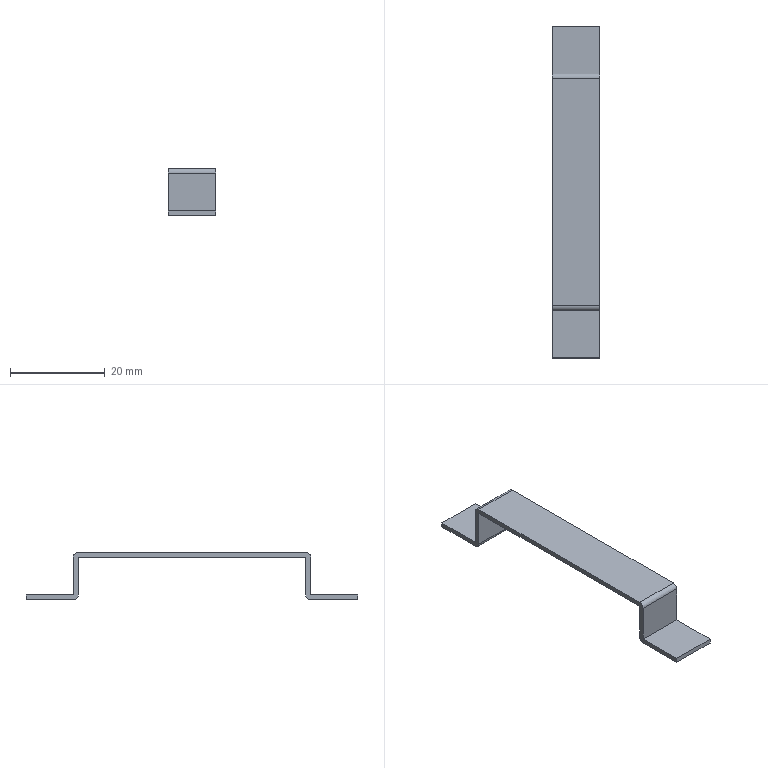Part | STEP file | RJWD-DY-0101_0002 | 1 solid | 18 faces | box 10 x 70 x 10 mm | volume 871.577 mm3 | plane 14 | cylinder 4 | commonest cylinder face diameters 2.004 x4
STEP:
#1=CARTESIAN_POINT('',(0.,0.,0.));
#2=DIRECTION('',(0.,0.,1.));
#3=DIRECTION('',(1.,0.,0.));
#4=AXIS2_PLACEMENT_3D('',#1,#2,#3);
#5=CARTESIAN_POINT('',(-540.773,5101.573,1740.644));
#6=VERTEX_POINT('',#5);
#7=CARTESIAN_POINT('',(-540.773,5101.573,1748.642));
#8=VERTEX_POINT('',#7);
#9=CARTESIAN_POINT('',(-540.773,5101.573,1740.644));
#10=DIRECTION('',(0.,-0.00008336,1.));
#11=VECTOR('',#10,1.);
#12=LINE('',#9,#11);
#13=CARTESIAN_POINT('',(-540.773,5101.573,1749.644));
#14=DIRECTION('',(1.,0.,0.));
#15=DIRECTION('',(0.,0.,-1.));
#16=AXIS2_PLACEMENT_3D('',#13,#14,#15);
#17=PLANE('',#16);
#18=CARTESIAN_POINT('',(8.999,0.0006667));
#19=DIRECTION('',(-1.,-0.00008336));
#20=VECTOR('',#19,1.);
#21=LINE('',#18,#20);
#22=(GEOMETRIC_REPRESENTATION_CONTEXT(2)PARAMETRIC_REPRESENTATION_CONTEXT()REPRESENTATION_CONTEXT('',''));
#23=DEFINITIONAL_REPRESENTATION('',(#21),#22);
#24=PCURVE('',#17,#23);
#25=CARTESIAN_POINT('',(0.,5101.573,0.));
#26=DIRECTION('',(0.,-1.,0.));
#27=DIRECTION('',(0.,0.,-1.));
#28=AXIS2_PLACEMENT_3D('',#25,#26,#27);
#29=PLANE('',#28);
#30=CARTESIAN_POINT('',(-1740.644,-540.773));
#31=DIRECTION('',(-1.,0.));
#32=VECTOR('',#31,1.);
#33=LINE('',#30,#32);
#34=(GEOMETRIC_REPRESENTATION_CONTEXT(2)PARAMETRIC_REPRESENTATION_CONTEXT()REPRESENTATION_CONTEXT('',''));
#35=DEFINITIONAL_REPRESENTATION('',(#33),#34);
#36=PCURVE('',#29,#35);
#37=SURFACE_CURVE('',#12,(#24,#36),.PCURVE_S1.);
#38=EDGE_CURVE('',#6,#8,#37,.T.);
#39=ORIENTED_EDGE('',*,*,#38,.T.);
#40=CARTESIAN_POINT('',(-540.773,5100.571,1749.644));
#41=VERTEX_POINT('',#40);
#42=CARTESIAN_POINT('',(-540.773,5100.571,1748.642));
#43=DIRECTION('',(-1.,0.,0.));
#44=DIRECTION('',(0.,0.,1.));
#45=AXIS2_PLACEMENT_3D('',#42,#43,#44);
#46=CIRCLE('',#45,1.002);
#47=CARTESIAN_POINT('',(0.,-1.002));
#48=CARTESIAN_POINT('',(0.,0.7335));
#49=CARTESIAN_POINT('',(1.503,-0.1342));
#50=CARTESIAN_POINT('',(3.006,-1.002));
#51=CARTESIAN_POINT('',(1.503,-1.87));
#52=CARTESIAN_POINT('',(0.,-2.738));
#53=CARTESIAN_POINT('',(0.,-1.002));
#54=(BOUNDED_CURVE()B_SPLINE_CURVE(2,(#47,#48,#49,#50,#51,#52,#53),.UNSPECIFIED.,.T.,.F.)B_SPLINE_CURVE_WITH_KNOTS((1,2,2,2,2,1),(-2.094,0.,2.094,4.189,6.283,8.378),.UNSPECIFIED.)CURVE()GEOMETRIC_REPRESENTATION_ITEM()RATIONAL_B_SPLINE_CURVE((1.,0.5,1.,0.5,1.,0.5,1.))REPRESENTATION_ITEM(''));
#55=(GEOMETRIC_REPRESENTATION_CONTEXT(2)PARAMETRIC_REPRESENTATION_CONTEXT()REPRESENTATION_CONTEXT('',''));
#56=DEFINITIONAL_REPRESENTATION('',(#54),#55);
#57=PCURVE('',#17,#56);
#58=CARTESIAN_POINT('',(-530.773,5100.571,1748.642));
#59=DIRECTION('',(-1.,0.,0.));
#60=DIRECTION('',(0.,0.,-1.));
#61=AXIS2_PLACEMENT_3D('',#58,#59,#60);
#62=CYLINDRICAL_SURFACE('',#61,1.002);
#63=CARTESIAN_POINT('',(3.142,10.));
#64=DIRECTION('',(1.,0.));
#65=VECTOR('',#64,1.);
#66=LINE('',#63,#65);
#67=(GEOMETRIC_REPRESENTATION_CONTEXT(2)PARAMETRIC_REPRESENTATION_CONTEXT()REPRESENTATION_CONTEXT('',''));
#68=DEFINITIONAL_REPRESENTATION('',(#66),#67);
#69=PCURVE('',#62,#68);
#70=SURFACE_CURVE('',#46,(#57,#69),.PCURVE_S1.);
#71=EDGE_CURVE('',#41,#8,#70,.T.);
#72=ORIENTED_EDGE('',*,*,#71,.F.);
#73=CARTESIAN_POINT('',(-540.773,5052.575,1749.644));
#74=VERTEX_POINT('',#73);
#75=CARTESIAN_POINT('',(-540.773,5052.575,1749.644));
#76=DIRECTION('',(0.,1.,0.));
#77=VECTOR('',#76,1.);
#78=LINE('',#75,#77);
#79=CARTESIAN_POINT('',(0.,-48.998));
#80=DIRECTION('',(0.,1.));
#81=VECTOR('',#80,1.);
#82=LINE('',#79,#81);
#83=(GEOMETRIC_REPRESENTATION_CONTEXT(2)PARAMETRIC_REPRESENTATION_CONTEXT()REPRESENTATION_CONTEXT('',''));
#84=DEFINITIONAL_REPRESENTATION('',(#82),#83);
#85=PCURVE('',#17,#84);
#86=CARTESIAN_POINT('',(0.,-600.,1749.644));
#87=DIRECTION('',(0.,0.,1.));
#88=DIRECTION('',(1.,0.,0.));
#89=AXIS2_PLACEMENT_3D('',#86,#87,#88);
#90=PLANE('',#89);
#91=CARTESIAN_POINT('',(-540.773,5652.575));
#92=DIRECTION('',(0.,1.));
#93=VECTOR('',#92,1.);
#94=LINE('',#91,#93);
#95=(GEOMETRIC_REPRESENTATION_CONTEXT(2)PARAMETRIC_REPRESENTATION_CONTEXT()REPRESENTATION_CONTEXT('',''));
#96=DEFINITIONAL_REPRESENTATION('',(#94),#95);
#97=PCURVE('',#90,#96);
#98=SURFACE_CURVE('',#78,(#85,#97),.PCURVE_S1.);
#99=EDGE_CURVE('',#74,#41,#98,.T.);
#100=ORIENTED_EDGE('',*,*,#99,.F.);
#101=CARTESIAN_POINT('',(-540.773,5051.573,1748.642));
#102=VERTEX_POINT('',#101);
#103=CARTESIAN_POINT('',(-540.773,5052.575,1748.642));
#104=DIRECTION('',(-1.,0.,0.));
#105=DIRECTION('',(0.,-1.,0.));
#106=AXIS2_PLACEMENT_3D('',#103,#104,#105);
#107=CIRCLE('',#106,1.002);
#108=CARTESIAN_POINT('',(1.002,-50.));
#109=CARTESIAN_POINT('',(-0.7335,-50.));
#110=CARTESIAN_POINT('',(0.1342,-48.497));
#111=CARTESIAN_POINT('',(1.002,-46.994));
#112=CARTESIAN_POINT('',(1.87,-48.497));
#113=CARTESIAN_POINT('',(2.738,-50.));
#114=CARTESIAN_POINT('',(1.002,-50.));
#115=(BOUNDED_CURVE()B_SPLINE_CURVE(2,(#108,#109,#110,#111,#112,#113,#114),.UNSPECIFIED.,.T.,.F.)B_SPLINE_CURVE_WITH_KNOTS((1,2,2,2,2,1),(-2.094,0.,2.094,4.189,6.283,8.378),.UNSPECIFIED.)CURVE()GEOMETRIC_REPRESENTATION_ITEM()RATIONAL_B_SPLINE_CURVE((1.,0.5,1.,0.5,1.,0.5,1.))REPRESENTATION_ITEM(''));
#116=(GEOMETRIC_REPRESENTATION_CONTEXT(2)PARAMETRIC_REPRESENTATION_CONTEXT()REPRESENTATION_CONTEXT('',''));
#117=DEFINITIONAL_REPRESENTATION('',(#115),#116);
#118=PCURVE('',#17,#117);
#119=CARTESIAN_POINT('',(-540.773,5052.575,1748.642));
#120=DIRECTION('',(1.,0.,0.));
#121=DIRECTION('',(0.,0.,-1.));
#122=AXIS2_PLACEMENT_3D('',#119,#120,#121);
#123=CYLINDRICAL_SURFACE('',#122,1.002);
#124=CARTESIAN_POINT('',(4.712,0.));
#125=DIRECTION('',(-1.,0.));
#126=VECTOR('',#125,1.);
#127=LINE('',#124,#126);
#128=(GEOMETRIC_REPRESENTATION_CONTEXT(2)PARAMETRIC_REPRESENTATION_CONTEXT()REPRESENTATION_CONTEXT('',''));
#129=DEFINITIONAL_REPRESENTATION('',(#127),#128);
#130=PCURVE('',#123,#129);
#131=SURFACE_CURVE('',#107,(#118,#130),.PCURVE_S1.);
#132=EDGE_CURVE('',#102,#74,#131,.T.);
#133=ORIENTED_EDGE('',*,*,#132,.F.);
#134=CARTESIAN_POINT('',(-540.773,5051.572,1740.644));
#135=VERTEX_POINT('',#134);
#136=CARTESIAN_POINT('',(-540.773,5051.572,1740.644));
#137=DIRECTION('',(0.,0.00008336,1.));
#138=VECTOR('',#137,1.);
#139=LINE('',#136,#138);
#140=CARTESIAN_POINT('',(8.999,-50.001));
#141=DIRECTION('',(-1.,0.00008336));
#142=VECTOR('',#141,1.);
#143=LINE('',#140,#142);
#144=(GEOMETRIC_REPRESENTATION_CONTEXT(2)PARAMETRIC_REPRESENTATION_CONTEXT()REPRESENTATION_CONTEXT('',''));
#145=DEFINITIONAL_REPRESENTATION('',(#143),#144);
#146=PCURVE('',#17,#145);
#147=CARTESIAN_POINT('',(0.,5051.573,0.));
#148=DIRECTION('',(0.,-1.,0.));
#149=DIRECTION('',(0.,0.,-1.));
#150=AXIS2_PLACEMENT_3D('',#147,#148,#149);
#151=PLANE('',#150);
#152=CARTESIAN_POINT('',(-1740.644,-540.773));
#153=DIRECTION('',(-1.,0.));
#154=VECTOR('',#153,1.);
#155=LINE('',#152,#154);
#156=(GEOMETRIC_REPRESENTATION_CONTEXT(2)PARAMETRIC_REPRESENTATION_CONTEXT()REPRESENTATION_CONTEXT('',''));
#157=DEFINITIONAL_REPRESENTATION('',(#155),#156);
#158=PCURVE('',#151,#157);
#159=SURFACE_CURVE('',#139,(#146,#158),.PCURVE_S1.);
#160=EDGE_CURVE('',#135,#102,#159,.T.);
#161=ORIENTED_EDGE('',*,*,#160,.F.);
#162=CARTESIAN_POINT('',(-540.773,5041.573,1740.644));
#163=VERTEX_POINT('',#162);
#164=CARTESIAN_POINT('',(-540.773,5041.573,1740.644));
#165=DIRECTION('',(0.,1.,0.00006667));
#166=VECTOR('',#165,1.);
#167=LINE('',#164,#166);
#168=CARTESIAN_POINT('',(9.,-60.));
#169=DIRECTION('',(-0.00006667,1.));
#170=VECTOR('',#169,1.);
#171=LINE('',#168,#170);
#172=(GEOMETRIC_REPRESENTATION_CONTEXT(2)PARAMETRIC_REPRESENTATION_CONTEXT()REPRESENTATION_CONTEXT('',''));
#173=DEFINITIONAL_REPRESENTATION('',(#171),#172);
#174=PCURVE('',#17,#173);
#175=CARTESIAN_POINT('',(0.,-600.,1740.644));
#176=DIRECTION('',(0.,0.,1.));
#177=DIRECTION('',(1.,0.,0.));
#178=AXIS2_PLACEMENT_3D('',#175,#176,#177);
#179=PLANE('',#178);
#180=CARTESIAN_POINT('',(-540.773,5641.573));
#181=DIRECTION('',(0.,1.));
#182=VECTOR('',#181,1.);
#183=LINE('',#180,#182);
#184=(GEOMETRIC_REPRESENTATION_CONTEXT(2)PARAMETRIC_REPRESENTATION_CONTEXT()REPRESENTATION_CONTEXT('',''));
#185=DEFINITIONAL_REPRESENTATION('',(#183),#184);
#186=PCURVE('',#179,#185);
#187=SURFACE_CURVE('',#167,(#174,#186),.PCURVE_S1.);
#188=EDGE_CURVE('',#163,#135,#187,.T.);
#189=ORIENTED_EDGE('',*,*,#188,.F.);
#190=CARTESIAN_POINT('',(-540.773,5041.573,1739.644));
#191=VERTEX_POINT('',#190);
#192=CARTESIAN_POINT('',(-540.773,5041.573,1740.644));
#193=DIRECTION('',(0.,0.,-1.));
#194=VECTOR('',#193,1.);
#195=LINE('',#192,#194);
#196=CARTESIAN_POINT('',(9.,-60.));
#197=DIRECTION('',(1.,0.));
#198=VECTOR('',#197,1.);
#199=LINE('',#196,#198);
#200=(GEOMETRIC_REPRESENTATION_CONTEXT(2)PARAMETRIC_REPRESENTATION_CONTEXT()REPRESENTATION_CONTEXT('',''));
#201=DEFINITIONAL_REPRESENTATION('',(#199),#200);
#202=PCURVE('',#17,#201);
#203=CARTESIAN_POINT('',(-540.773,5041.573,1739.644));
#204=DIRECTION('',(0.,-1.,0.));
#205=DIRECTION('',(0.,0.,-1.));
#206=AXIS2_PLACEMENT_3D('',#203,#204,#205);
#207=PLANE('',#206);
#208=CARTESIAN_POINT('',(-1.,0.));
#209=DIRECTION('',(1.,0.));
#210=VECTOR('',#209,1.);
#211=LINE('',#208,#210);
#212=(GEOMETRIC_REPRESENTATION_CONTEXT(2)PARAMETRIC_REPRESENTATION_CONTEXT()REPRESENTATION_CONTEXT('',''));
#213=DEFINITIONAL_REPRESENTATION('',(#211),#212);
#214=PCURVE('',#207,#213);
#215=SURFACE_CURVE('',#195,(#202,#214),.PCURVE_S1.);
#216=EDGE_CURVE('',#163,#191,#215,.T.);
#217=ORIENTED_EDGE('',*,*,#216,.T.);
#218=CARTESIAN_POINT('',(-540.773,5051.571,1739.644));
#219=VERTEX_POINT('',#218);
#220=CARTESIAN_POINT('',(-540.773,5041.573,1739.644));
#221=DIRECTION('',(0.,1.,0.));
#222=VECTOR('',#221,1.);
#223=LINE('',#220,#222);
#224=CARTESIAN_POINT('',(10.,-60.));
#225=DIRECTION('',(0.,1.));
#226=VECTOR('',#225,1.);
#227=LINE('',#224,#226);
#228=(GEOMETRIC_REPRESENTATION_CONTEXT(2)PARAMETRIC_REPRESENTATION_CONTEXT()REPRESENTATION_CONTEXT('',''));
#229=DEFINITIONAL_REPRESENTATION('',(#227),#228);
#230=PCURVE('',#17,#229);
#231=CARTESIAN_POINT('',(0.,-600.,1739.644));
#232=DIRECTION('',(0.,0.,1.));
#233=DIRECTION('',(1.,0.,0.));
#234=AXIS2_PLACEMENT_3D('',#231,#232,#233);
#235=PLANE('',#234);
#236=CARTESIAN_POINT('',(-540.773,5641.573));
#237=DIRECTION('',(0.,1.));
#238=VECTOR('',#237,1.);
#239=LINE('',#236,#238);
#240=(GEOMETRIC_REPRESENTATION_CONTEXT(2)PARAMETRIC_REPRESENTATION_CONTEXT()REPRESENTATION_CONTEXT('',''));
#241=DEFINITIONAL_REPRESENTATION('',(#239),#240);
#242=PCURVE('',#235,#241);
#243=SURFACE_CURVE('',#223,(#230,#242),.PCURVE_S1.);
#244=EDGE_CURVE('',#191,#219,#243,.T.);
#245=ORIENTED_EDGE('',*,*,#244,.T.);
#246=CARTESIAN_POINT('',(-540.773,5052.573,1740.646));
#247=VERTEX_POINT('',#246);
#248=CARTESIAN_POINT('',(-540.773,5051.571,1740.646));
#249=DIRECTION('',(-1.,0.,0.));
#250=DIRECTION('',(0.,1.,0.));
#251=AXIS2_PLACEMENT_3D('',#248,#249,#250);
#252=CIRCLE('',#251,1.002);
#253=CARTESIAN_POINT('',(8.998,-49.));
#254=CARTESIAN_POINT('',(10.734,-49.));
#255=CARTESIAN_POINT('',(9.866,-50.503));
#256=CARTESIAN_POINT('',(8.998,-52.006));
#257=CARTESIAN_POINT('',(8.13,-50.503));
#258=CARTESIAN_POINT('',(7.262,-49.));
#259=CARTESIAN_POINT('',(8.998,-49.));
#260=(BOUNDED_CURVE()B_SPLINE_CURVE(2,(#253,#254,#255,#256,#257,#258,#259),.UNSPECIFIED.,.T.,.F.)B_SPLINE_CURVE_WITH_KNOTS((1,2,2,2,2,1),(-2.094,0.,2.094,4.189,6.283,8.378),.UNSPECIFIED.)CURVE()GEOMETRIC_REPRESENTATION_ITEM()RATIONAL_B_SPLINE_CURVE((1.,0.5,1.,0.5,1.,0.5,1.))REPRESENTATION_ITEM(''));
#261=(GEOMETRIC_REPRESENTATION_CONTEXT(2)PARAMETRIC_REPRESENTATION_CONTEXT()REPRESENTATION_CONTEXT('',''));
#262=DEFINITIONAL_REPRESENTATION('',(#260),#261);
#263=PCURVE('',#17,#262);
#264=CARTESIAN_POINT('',(-530.773,5051.571,1740.646));
#265=DIRECTION('',(-1.,0.,0.));
#266=DIRECTION('',(0.,-1.,0.));
#267=AXIS2_PLACEMENT_3D('',#264,#265,#266);
#268=CYLINDRICAL_SURFACE('',#267,1.002);
#269=CARTESIAN_POINT('',(3.142,10.));
#270=DIRECTION('',(1.,0.));
#271=VECTOR('',#270,1.);
#272=LINE('',#269,#271);
#273=(GEOMETRIC_REPRESENTATION_CONTEXT(2)PARAMETRIC_REPRESENTATION_CONTEXT()REPRESENTATION_CONTEXT('',''));
#274=DEFINITIONAL_REPRESENTATION('',(#272),#273);
#275=PCURVE('',#268,#274);
#276=SURFACE_CURVE('',#252,(#263,#275),.PCURVE_S1.);
#277=EDGE_CURVE('',#247,#219,#276,.T.);
#278=ORIENTED_EDGE('',*,*,#277,.F.);
#279=CARTESIAN_POINT('',(-540.773,5052.573,1748.643));
#280=VERTEX_POINT('',#279);
#281=CARTESIAN_POINT('',(-540.773,5052.573,1740.646));
#282=DIRECTION('',(0.,0.00008336,1.));
#283=VECTOR('',#282,1.);
#284=LINE('',#281,#283);
#285=CARTESIAN_POINT('',(8.998,-49.));
#286=DIRECTION('',(-1.,0.00008336));
#287=VECTOR('',#286,1.);
#288=LINE('',#285,#287);
#289=(GEOMETRIC_REPRESENTATION_CONTEXT(2)PARAMETRIC_REPRESENTATION_CONTEXT()REPRESENTATION_CONTEXT('',''));
#290=DEFINITIONAL_REPRESENTATION('',(#288),#289);
#291=PCURVE('',#17,#290);
#292=CARTESIAN_POINT('',(0.,5052.573,0.));
#293=DIRECTION('',(0.,-1.,0.));
#294=DIRECTION('',(0.,0.,-1.));
#295=AXIS2_PLACEMENT_3D('',#292,#293,#294);
#296=PLANE('',#295);
#297=CARTESIAN_POINT('',(-1740.646,-540.773));
#298=DIRECTION('',(-1.,0.));
#299=VECTOR('',#298,1.);
#300=LINE('',#297,#299);
#301=(GEOMETRIC_REPRESENTATION_CONTEXT(2)PARAMETRIC_REPRESENTATION_CONTEXT()REPRESENTATION_CONTEXT('',''));
#302=DEFINITIONAL_REPRESENTATION('',(#300),#301);
#303=PCURVE('',#296,#302);
#304=SURFACE_CURVE('',#284,(#291,#303),.PCURVE_S1.);
#305=EDGE_CURVE('',#247,#280,#304,.T.);
#306=ORIENTED_EDGE('',*,*,#305,.T.);
#307=CARTESIAN_POINT('',(-540.773,5100.572,1748.643));
#308=VERTEX_POINT('',#307);
#309=CARTESIAN_POINT('',(-540.773,5052.573,1748.643));
#310=DIRECTION('',(0.,1.,0.));
#311=VECTOR('',#310,1.);
#312=LINE('',#309,#311);
#313=CARTESIAN_POINT('',(1.001,-48.999));
#314=DIRECTION('',(0.,1.));
#315=VECTOR('',#314,1.);
#316=LINE('',#313,#315);
#317=(GEOMETRIC_REPRESENTATION_CONTEXT(2)PARAMETRIC_REPRESENTATION_CONTEXT()REPRESENTATION_CONTEXT('',''));
#318=DEFINITIONAL_REPRESENTATION('',(#316),#317);
#319=PCURVE('',#17,#318);
#320=CARTESIAN_POINT('',(0.,-600.,1748.644));
#321=DIRECTION('',(0.,0.,1.));
#322=DIRECTION('',(1.,0.,0.));
#323=AXIS2_PLACEMENT_3D('',#320,#321,#322);
#324=PLANE('',#323);
#325=CARTESIAN_POINT('',(-540.773,5652.573));
#326=DIRECTION('',(0.,1.));
#327=VECTOR('',#326,1.);
#328=LINE('',#325,#327);
#329=(GEOMETRIC_REPRESENTATION_CONTEXT(2)PARAMETRIC_REPRESENTATION_CONTEXT()REPRESENTATION_CONTEXT('',''));
#330=DEFINITIONAL_REPRESENTATION('',(#328),#329);
#331=PCURVE('',#324,#330);
#332=SURFACE_CURVE('',#312,(#319,#331),.PCURVE_S1.);
#333=EDGE_CURVE('',#280,#308,#332,.T.);
#334=ORIENTED_EDGE('',*,*,#333,.T.);
#335=CARTESIAN_POINT('',(-540.773,5100.573,1740.646));
#336=VERTEX_POINT('',#335);
#337=CARTESIAN_POINT('',(-540.773,5100.573,1740.646));
#338=DIRECTION('',(0.,-0.00008336,1.));
#339=VECTOR('',#338,1.);
#340=LINE('',#337,#339);
#341=CARTESIAN_POINT('',(8.998,-1.));
#342=DIRECTION('',(-1.,-0.00008336));
#343=VECTOR('',#342,1.);
#344=LINE('',#341,#343);
#345=(GEOMETRIC_REPRESENTATION_CONTEXT(2)PARAMETRIC_REPRESENTATION_CONTEXT()REPRESENTATION_CONTEXT('',''));
#346=DEFINITIONAL_REPRESENTATION('',(#344),#345);
#347=PCURVE('',#17,#346);
#348=CARTESIAN_POINT('',(0.,5100.573,0.));
#349=DIRECTION('',(0.,-1.,0.));
#350=DIRECTION('',(0.,0.,-1.));
#351=AXIS2_PLACEMENT_3D('',#348,#349,#350);
#352=PLANE('',#351);
#353=CARTESIAN_POINT('',(-1740.646,-540.773));
#354=DIRECTION('',(-1.,0.));
#355=VECTOR('',#354,1.);
#356=LINE('',#353,#355);
#357=(GEOMETRIC_REPRESENTATION_CONTEXT(2)PARAMETRIC_REPRESENTATION_CONTEXT()REPRESENTATION_CONTEXT('',''));
#358=DEFINITIONAL_REPRESENTATION('',(#356),#357);
#359=PCURVE('',#352,#358);
#360=SURFACE_CURVE('',#340,(#347,#359),.PCURVE_S1.);
#361=EDGE_CURVE('',#336,#308,#360,.T.);
#362=ORIENTED_EDGE('',*,*,#361,.F.);
#363=CARTESIAN_POINT('',(-540.773,5101.575,1739.644));
#364=VERTEX_POINT('',#363);
#365=CARTESIAN_POINT('',(-540.773,5101.575,1740.646));
#366=DIRECTION('',(-1.,0.,0.));
#367=DIRECTION('',(0.,0.,-1.));
#368=AXIS2_PLACEMENT_3D('',#365,#366,#367);
#369=CIRCLE('',#368,1.002);
#370=CARTESIAN_POINT('',(10.,0.002));
#371=CARTESIAN_POINT('',(10.,-1.734));
#372=CARTESIAN_POINT('',(8.497,-0.8658));
#373=CARTESIAN_POINT('',(6.994,0.002));
#374=CARTESIAN_POINT('',(8.497,0.8698));
#375=CARTESIAN_POINT('',(10.,1.738));
#376=CARTESIAN_POINT('',(10.,0.002));
#377=(BOUNDED_CURVE()B_SPLINE_CURVE(2,(#370,#371,#372,#373,#374,#375,#376),.UNSPECIFIED.,.T.,.F.)B_SPLINE_CURVE_WITH_KNOTS((1,2,2,2,2,1),(-2.094,0.,2.094,4.189,6.283,8.378),.UNSPECIFIED.)CURVE()GEOMETRIC_REPRESENTATION_ITEM()RATIONAL_B_SPLINE_CURVE((1.,0.5,1.,0.5,1.,0.5,1.))REPRESENTATION_ITEM(''));
#378=(GEOMETRIC_REPRESENTATION_CONTEXT(2)PARAMETRIC_REPRESENTATION_CONTEXT()REPRESENTATION_CONTEXT('',''));
#379=DEFINITIONAL_REPRESENTATION('',(#377),#378);
#380=PCURVE('',#17,#379);
#381=CARTESIAN_POINT('',(-540.773,5101.575,1740.646));
#382=DIRECTION('',(1.,0.,0.));
#383=DIRECTION('',(0.,1.,0.));
#384=AXIS2_PLACEMENT_3D('',#381,#382,#383);
#385=CYLINDRICAL_SURFACE('',#384,1.002);
#386=CARTESIAN_POINT('',(4.712,0.));
#387=DIRECTION('',(-1.,0.));
#388=VECTOR('',#387,1.);
#389=LINE('',#386,#388);
#390=(GEOMETRIC_REPRESENTATION_CONTEXT(2)PARAMETRIC_REPRESENTATION_CONTEXT()REPRESENTATION_CONTEXT('',''));
#391=DEFINITIONAL_REPRESENTATION('',(#389),#390);
#392=PCURVE('',#385,#391);
#393=SURFACE_CURVE('',#369,(#380,#392),.PCURVE_S1.);
#394=EDGE_CURVE('',#364,#336,#393,.T.);
#395=ORIENTED_EDGE('',*,*,#394,.F.);
#396=CARTESIAN_POINT('',(-540.773,5111.573,1739.644));
#397=VERTEX_POINT('',#396);
#398=CARTESIAN_POINT('',(-540.773,5111.573,1739.644));
#399=DIRECTION('',(0.,-1.,0.));
#400=VECTOR('',#399,1.);
#401=LINE('',#398,#400);
#402=CARTESIAN_POINT('',(10.,10.));
#403=DIRECTION('',(0.,-1.));
#404=VECTOR('',#403,1.);
#405=LINE('',#402,#404);
#406=(GEOMETRIC_REPRESENTATION_CONTEXT(2)PARAMETRIC_REPRESENTATION_CONTEXT()REPRESENTATION_CONTEXT('',''));
#407=DEFINITIONAL_REPRESENTATION('',(#405),#406);
#408=PCURVE('',#17,#407);
#409=CARTESIAN_POINT('',(0.,-600.,1739.644));
#410=DIRECTION('',(0.,0.,-1.));
#411=DIRECTION('',(-1.,0.,0.));
#412=AXIS2_PLACEMENT_3D('',#409,#410,#411);
#413=PLANE('',#412);
#414=CARTESIAN_POINT('',(540.773,5711.573));
#415=DIRECTION('',(0.,-1.));
#416=VECTOR('',#415,1.);
#417=LINE('',#414,#416);
#418=(GEOMETRIC_REPRESENTATION_CONTEXT(2)PARAMETRIC_REPRESENTATION_CONTEXT()REPRESENTATION_CONTEXT('',''));
#419=DEFINITIONAL_REPRESENTATION('',(#417),#418);
#420=PCURVE('',#413,#419);
#421=SURFACE_CURVE('',#401,(#408,#420),.PCURVE_S1.);
#422=EDGE_CURVE('',#397,#364,#421,.T.);
#423=ORIENTED_EDGE('',*,*,#422,.F.);
#424=CARTESIAN_POINT('',(-540.773,5111.573,1740.644));
#425=VERTEX_POINT('',#424);
#426=CARTESIAN_POINT('',(-540.773,5111.573,1740.644));
#427=DIRECTION('',(0.,0.,-1.));
#428=VECTOR('',#427,1.);
#429=LINE('',#426,#428);
#430=CARTESIAN_POINT('',(9.,10.));
#431=DIRECTION('',(1.,0.));
#432=VECTOR('',#431,1.);
#433=LINE('',#430,#432);
#434=(GEOMETRIC_REPRESENTATION_CONTEXT(2)PARAMETRIC_REPRESENTATION_CONTEXT()REPRESENTATION_CONTEXT('',''));
#435=DEFINITIONAL_REPRESENTATION('',(#433),#434);
#436=PCURVE('',#17,#435);
#437=CARTESIAN_POINT('',(-540.773,5111.573,1739.644));
#438=DIRECTION('',(0.,-1.,0.));
#439=DIRECTION('',(0.,0.,-1.));
#440=AXIS2_PLACEMENT_3D('',#437,#438,#439);
#441=PLANE('',#440);
#442=CARTESIAN_POINT('',(-1.,0.));
#443=DIRECTION('',(1.,0.));
#444=VECTOR('',#443,1.);
#445=LINE('',#442,#444);
#446=(GEOMETRIC_REPRESENTATION_CONTEXT(2)PARAMETRIC_REPRESENTATION_CONTEXT()REPRESENTATION_CONTEXT('',''));
#447=DEFINITIONAL_REPRESENTATION('',(#445),#446);
#448=PCURVE('',#441,#447);
#449=SURFACE_CURVE('',#429,(#436,#448),.PCURVE_S1.);
#450=EDGE_CURVE('',#425,#397,#449,.T.);
#451=ORIENTED_EDGE('',*,*,#450,.F.);
#452=CARTESIAN_POINT('',(-540.773,5111.573,1740.644));
#453=DIRECTION('',(0.,-1.,0.00006667));
#454=VECTOR('',#453,1.);
#455=LINE('',#452,#454);
#456=CARTESIAN_POINT('',(9.,10.));
#457=DIRECTION('',(-0.00006667,-1.));
#458=VECTOR('',#457,1.);
#459=LINE('',#456,#458);
#460=(GEOMETRIC_REPRESENTATION_CONTEXT(2)PARAMETRIC_REPRESENTATION_CONTEXT()REPRESENTATION_CONTEXT('',''));
#461=DEFINITIONAL_REPRESENTATION('',(#459),#460);
#462=PCURVE('',#17,#461);
#463=CARTESIAN_POINT('',(0.,-600.,1740.644));
#464=DIRECTION('',(0.,0.,-1.));
#465=DIRECTION('',(-1.,0.,0.));
#466=AXIS2_PLACEMENT_3D('',#463,#464,#465);
#467=PLANE('',#466);
#468=CARTESIAN_POINT('',(540.773,5711.573));
#469=DIRECTION('',(0.,-1.));
#470=VECTOR('',#469,1.);
#471=LINE('',#468,#470);
#472=(GEOMETRIC_REPRESENTATION_CONTEXT(2)PARAMETRIC_REPRESENTATION_CONTEXT()REPRESENTATION_CONTEXT('',''));
#473=DEFINITIONAL_REPRESENTATION('',(#471),#472);
#474=PCURVE('',#467,#473);
#475=SURFACE_CURVE('',#455,(#462,#474),.PCURVE_S1.);
#476=EDGE_CURVE('',#425,#6,#475,.T.);
#477=ORIENTED_EDGE('',*,*,#476,.T.);
#478=EDGE_LOOP('',(#39,#72,#100,#133,#161,#189,#217,#245,#278,#306,#334,#362,#395,#423,#451,#477));
#479=FACE_BOUND('',#478,.F.);
#480=ADVANCED_FACE('',(#479),#17,.F.);
#481=CARTESIAN_POINT('',(-530.773,5101.573,1740.644));
#482=VERTEX_POINT('',#481);
#483=CARTESIAN_POINT('',(-540.773,5101.573,1740.644));
#484=DIRECTION('',(1.,0.,0.));
#485=VECTOR('',#484,1.);
#486=LINE('',#483,#485);
#487=CARTESIAN_POINT('',(-1740.644,-540.773));
#488=DIRECTION('',(0.,1.));
#489=VECTOR('',#488,1.);
#490=LINE('',#487,#489);
#491=(GEOMETRIC_REPRESENTATION_CONTEXT(2)PARAMETRIC_REPRESENTATION_CONTEXT()REPRESENTATION_CONTEXT('',''));
#492=DEFINITIONAL_REPRESENTATION('',(#490),#491);
#493=PCURVE('',#29,#492);
#494=CARTESIAN_POINT('',(540.773,5701.573));
#495=DIRECTION('',(-1.,0.));
#496=VECTOR('',#495,1.);
#497=LINE('',#494,#496);
#498=(GEOMETRIC_REPRESENTATION_CONTEXT(2)PARAMETRIC_REPRESENTATION_CONTEXT()REPRESENTATION_CONTEXT('',''));
#499=DEFINITIONAL_REPRESENTATION('',(#497),#498);
#500=PCURVE('',#467,#499);
#501=SURFACE_CURVE('',#486,(#493,#500),.PCURVE_S1.);
#502=EDGE_CURVE('',#6,#482,#501,.T.);
#503=ORIENTED_EDGE('',*,*,#502,.T.);
#504=CARTESIAN_POINT('',(-530.773,5101.573,1748.642));
#505=VERTEX_POINT('',#504);
#506=CARTESIAN_POINT('',(-530.773,5101.573,1748.642));
#507=DIRECTION('',(0.,0.00008336,-1.));
#508=VECTOR('',#507,1.);
#509=LINE('',#506,#508);
#510=CARTESIAN_POINT('',(-1748.642,-530.773));
#511=DIRECTION('',(1.,0.));
#512=VECTOR('',#511,1.);
#513=LINE('',#510,#512);
#514=(GEOMETRIC_REPRESENTATION_CONTEXT(2)PARAMETRIC_REPRESENTATION_CONTEXT()REPRESENTATION_CONTEXT('',''));
#515=DEFINITIONAL_REPRESENTATION('',(#513),#514);
#516=PCURVE('',#29,#515);
#517=CARTESIAN_POINT('',(-530.773,5051.573,1749.644));
#518=DIRECTION('',(-1.,0.,0.));
#519=DIRECTION('',(0.,0.,1.));
#520=AXIS2_PLACEMENT_3D('',#517,#518,#519);
#521=PLANE('',#520);
#522=CARTESIAN_POINT('',(-1.002,50.));
#523=DIRECTION('',(-1.,0.00008336));
#524=VECTOR('',#523,1.);
#525=LINE('',#522,#524);
#526=(GEOMETRIC_REPRESENTATION_CONTEXT(2)PARAMETRIC_REPRESENTATION_CONTEXT()REPRESENTATION_CONTEXT('',''));
#527=DEFINITIONAL_REPRESENTATION('',(#525),#526);
#528=PCURVE('',#521,#527);
#529=SURFACE_CURVE('',#509,(#516,#528),.PCURVE_S1.);
#530=EDGE_CURVE('',#505,#482,#529,.T.);
#531=ORIENTED_EDGE('',*,*,#530,.F.);
#532=CARTESIAN_POINT('',(-530.773,5101.573,1748.642));
#533=DIRECTION('',(-1.,0.,0.));
#534=VECTOR('',#533,1.);
#535=LINE('',#532,#534);
#536=CARTESIAN_POINT('',(-1748.642,-530.773));
#537=DIRECTION('',(0.,-1.));
#538=VECTOR('',#537,1.);
#539=LINE('',#536,#538);
#540=(GEOMETRIC_REPRESENTATION_CONTEXT(2)PARAMETRIC_REPRESENTATION_CONTEXT()REPRESENTATION_CONTEXT('',''));
#541=DEFINITIONAL_REPRESENTATION('',(#539),#540);
#542=PCURVE('',#29,#541);
#543=CARTESIAN_POINT('',(4.712,0.));
#544=DIRECTION('',(0.,1.));
#545=VECTOR('',#544,1.);
#546=LINE('',#543,#545);
#547=(GEOMETRIC_REPRESENTATION_CONTEXT(2)PARAMETRIC_REPRESENTATION_CONTEXT()REPRESENTATION_CONTEXT('',''));
#548=DEFINITIONAL_REPRESENTATION('',(#546),#547);
#549=PCURVE('',#62,#548);
#550=SURFACE_CURVE('',#535,(#542,#549),.PCURVE_S1.);
#551=EDGE_CURVE('',#505,#8,#550,.T.);
#552=ORIENTED_EDGE('',*,*,#551,.T.);
#553=ORIENTED_EDGE('',*,*,#38,.F.);
#554=EDGE_LOOP('',(#503,#531,#552,#553));
#555=FACE_BOUND('',#554,.F.);
#556=ADVANCED_FACE('',(#555),#29,.F.);
#557=ORIENTED_EDGE('',*,*,#502,.F.);
#558=ORIENTED_EDGE('',*,*,#476,.F.);
#559=CARTESIAN_POINT('',(-530.773,5111.573,1740.644));
#560=VERTEX_POINT('',#559);
#561=CARTESIAN_POINT('',(-530.773,5111.573,1740.644));
#562=DIRECTION('',(-1.,0.,0.));
#563=VECTOR('',#562,1.);
#564=LINE('',#561,#563);
#565=CARTESIAN_POINT('',(530.773,5711.573));
#566=DIRECTION('',(1.,0.));
#567=VECTOR('',#566,1.);
#568=LINE('',#565,#567);
#569=(GEOMETRIC_REPRESENTATION_CONTEXT(2)PARAMETRIC_REPRESENTATION_CONTEXT()REPRESENTATION_CONTEXT('',''));
#570=DEFINITIONAL_REPRESENTATION('',(#568),#569);
#571=PCURVE('',#467,#570);
#572=CARTESIAN_POINT('',(-1.,10.));
#573=DIRECTION('',(0.,-1.));
#574=VECTOR('',#573,1.);
#575=LINE('',#572,#574);
#576=(GEOMETRIC_REPRESENTATION_CONTEXT(2)PARAMETRIC_REPRESENTATION_CONTEXT()REPRESENTATION_CONTEXT('',''));
#577=DEFINITIONAL_REPRESENTATION('',(#575),#576);
#578=PCURVE('',#441,#577);
#579=SURFACE_CURVE('',#564,(#571,#578),.PCURVE_S1.);
#580=EDGE_CURVE('',#560,#425,#579,.T.);
#581=ORIENTED_EDGE('',*,*,#580,.F.);
#582=CARTESIAN_POINT('',(-530.773,5101.573,1740.644));
#583=DIRECTION('',(0.,1.,-0.00006667));
#584=VECTOR('',#583,1.);
#585=LINE('',#582,#584);
#586=CARTESIAN_POINT('',(530.773,5701.573));
#587=DIRECTION('',(0.,1.));
#588=VECTOR('',#587,1.);
#589=LINE('',#586,#588);
#590=(GEOMETRIC_REPRESENTATION_CONTEXT(2)PARAMETRIC_REPRESENTATION_CONTEXT()REPRESENTATION_CONTEXT('',''));
#591=DEFINITIONAL_REPRESENTATION('',(#589),#590);
#592=PCURVE('',#467,#591);
#593=CARTESIAN_POINT('',(-8.999,50.001));
#594=DIRECTION('',(-0.00006667,1.));
#595=VECTOR('',#594,1.);
#596=LINE('',#593,#595);
#597=(GEOMETRIC_REPRESENTATION_CONTEXT(2)PARAMETRIC_REPRESENTATION_CONTEXT()REPRESENTATION_CONTEXT('',''));
#598=DEFINITIONAL_REPRESENTATION('',(#596),#597);
#599=PCURVE('',#521,#598);
#600=SURFACE_CURVE('',#585,(#592,#599),.PCURVE_S1.);
#601=EDGE_CURVE('',#482,#560,#600,.T.);
#602=ORIENTED_EDGE('',*,*,#601,.F.);
#603=EDGE_LOOP('',(#557,#558,#581,#602));
#604=FACE_BOUND('',#603,.F.);
#605=ADVANCED_FACE('',(#604),#467,.F.);
#606=ORIENTED_EDGE('',*,*,#580,.T.);
#607=ORIENTED_EDGE('',*,*,#450,.T.);
#608=CARTESIAN_POINT('',(-530.773,5111.573,1739.644));
#609=VERTEX_POINT('',#608);
#610=CARTESIAN_POINT('',(-530.773,5111.573,1739.644));
#611=DIRECTION('',(-1.,0.,0.));
#612=VECTOR('',#611,1.);
#613=LINE('',#610,#612);
#614=CARTESIAN_POINT('',(0.,10.));
#615=DIRECTION('',(0.,-1.));
#616=VECTOR('',#615,1.);
#617=LINE('',#614,#616);
#618=(GEOMETRIC_REPRESENTATION_CONTEXT(2)PARAMETRIC_REPRESENTATION_CONTEXT()REPRESENTATION_CONTEXT('',''));
#619=DEFINITIONAL_REPRESENTATION('',(#617),#618);
#620=PCURVE('',#441,#619);
#621=CARTESIAN_POINT('',(530.773,5711.573));
#622=DIRECTION('',(1.,0.));
#623=VECTOR('',#622,1.);
#624=LINE('',#621,#623);
#625=(GEOMETRIC_REPRESENTATION_CONTEXT(2)PARAMETRIC_REPRESENTATION_CONTEXT()REPRESENTATION_CONTEXT('',''));
#626=DEFINITIONAL_REPRESENTATION('',(#624),#625);
#627=PCURVE('',#413,#626);
#628=SURFACE_CURVE('',#613,(#620,#627),.PCURVE_S1.);
#629=EDGE_CURVE('',#609,#397,#628,.T.);
#630=ORIENTED_EDGE('',*,*,#629,.F.);
#631=CARTESIAN_POINT('',(-530.773,5111.573,1740.644));
#632=DIRECTION('',(0.,0.,-1.));
#633=VECTOR('',#632,1.);
#634=LINE('',#631,#633);
#635=CARTESIAN_POINT('',(-1.,10.));
#636=DIRECTION('',(1.,0.));
#637=VECTOR('',#636,1.);
#638=LINE('',#635,#637);
#639=(GEOMETRIC_REPRESENTATION_CONTEXT(2)PARAMETRIC_REPRESENTATION_CONTEXT()REPRESENTATION_CONTEXT('',''));
#640=DEFINITIONAL_REPRESENTATION('',(#638),#639);
#641=PCURVE('',#441,#640);
#642=CARTESIAN_POINT('',(-9.,60.));
#643=DIRECTION('',(-1.,0.));
#644=VECTOR('',#643,1.);
#645=LINE('',#642,#644);
#646=(GEOMETRIC_REPRESENTATION_CONTEXT(2)PARAMETRIC_REPRESENTATION_CONTEXT()REPRESENTATION_CONTEXT('',''));
#647=DEFINITIONAL_REPRESENTATION('',(#645),#646);
#648=PCURVE('',#521,#647);
#649=SURFACE_CURVE('',#634,(#641,#648),.PCURVE_S1.);
#650=EDGE_CURVE('',#560,#609,#649,.T.);
#651=ORIENTED_EDGE('',*,*,#650,.F.);
#652=EDGE_LOOP('',(#606,#607,#630,#651));
#653=FACE_BOUND('',#652,.F.);
#654=ADVANCED_FACE('',(#653),#441,.F.);
#655=CARTESIAN_POINT('',(-530.773,5101.575,1739.644));
#656=VERTEX_POINT('',#655);
#657=CARTESIAN_POINT('',(-530.773,5101.575,1739.644));
#658=DIRECTION('',(0.,1.,0.));
#659=VECTOR('',#658,1.);
#660=LINE('',#657,#659);
#661=CARTESIAN_POINT('',(530.773,5701.575));
#662=DIRECTION('',(0.,1.));
#663=VECTOR('',#662,1.);
#664=LINE('',#661,#663);
#665=(GEOMETRIC_REPRESENTATION_CONTEXT(2)PARAMETRIC_REPRESENTATION_CONTEXT()REPRESENTATION_CONTEXT('',''));
#666=DEFINITIONAL_REPRESENTATION('',(#664),#665);
#667=PCURVE('',#413,#666);
#668=CARTESIAN_POINT('',(-10.,50.002));
#669=DIRECTION('',(0.,1.));
#670=VECTOR('',#669,1.);
#671=LINE('',#668,#670);
#672=(GEOMETRIC_REPRESENTATION_CONTEXT(2)PARAMETRIC_REPRESENTATION_CONTEXT()REPRESENTATION_CONTEXT('',''));
#673=DEFINITIONAL_REPRESENTATION('',(#671),#672);
#674=PCURVE('',#521,#673);
#675=SURFACE_CURVE('',#660,(#667,#674),.PCURVE_S1.);
#676=EDGE_CURVE('',#656,#609,#675,.T.);
#677=ORIENTED_EDGE('',*,*,#676,.T.);
#678=ORIENTED_EDGE('',*,*,#629,.T.);
#679=ORIENTED_EDGE('',*,*,#422,.T.);
#680=CARTESIAN_POINT('',(-540.773,5101.575,1739.644));
#681=DIRECTION('',(1.,0.,0.));
#682=VECTOR('',#681,1.);
#683=LINE('',#680,#682);
#684=CARTESIAN_POINT('',(540.773,5701.575));
#685=DIRECTION('',(-1.,0.));
#686=VECTOR('',#685,1.);
#687=LINE('',#684,#686);
#688=(GEOMETRIC_REPRESENTATION_CONTEXT(2)PARAMETRIC_REPRESENTATION_CONTEXT()REPRESENTATION_CONTEXT('',''));
#689=DEFINITIONAL_REPRESENTATION('',(#687),#688);
#690=PCURVE('',#413,#689);
#691=CARTESIAN_POINT('',(4.712,0.));
#692=DIRECTION('',(0.,1.));
#693=VECTOR('',#692,1.);
#694=LINE('',#691,#693);
#695=(GEOMETRIC_REPRESENTATION_CONTEXT(2)PARAMETRIC_REPRESENTATION_CONTEXT()REPRESENTATION_CONTEXT('',''));
#696=DEFINITIONAL_REPRESENTATION('',(#694),#695);
#697=PCURVE('',#385,#696);
#698=SURFACE_CURVE('',#683,(#690,#697),.PCURVE_S1.);
#699=EDGE_CURVE('',#364,#656,#698,.T.);
#700=ORIENTED_EDGE('',*,*,#699,.T.);
#701=EDGE_LOOP('',(#677,#678,#679,#700));
#702=FACE_BOUND('',#701,.F.);
#703=ADVANCED_FACE('',(#702),#413,.T.);
#704=CARTESIAN_POINT('',(-530.773,5100.572,1748.643));
#705=VERTEX_POINT('',#704);
#706=CARTESIAN_POINT('',(-530.773,5100.573,1740.646));
#707=VERTEX_POINT('',#706);
#708=CARTESIAN_POINT('',(-530.773,5100.572,1748.643));
#709=DIRECTION('',(0.,0.00008336,-1.));
#710=VECTOR('',#709,1.);
#711=LINE('',#708,#710);
#712=CARTESIAN_POINT('',(-1.001,48.999));
#713=DIRECTION('',(-1.,0.00008336));
#714=VECTOR('',#713,1.);
#715=LINE('',#712,#714);
#716=(GEOMETRIC_REPRESENTATION_CONTEXT(2)PARAMETRIC_REPRESENTATION_CONTEXT()REPRESENTATION_CONTEXT('',''));
#717=DEFINITIONAL_REPRESENTATION('',(#715),#716);
#718=PCURVE('',#521,#717);
#719=CARTESIAN_POINT('',(-1748.643,-530.773));
#720=DIRECTION('',(1.,0.));
#721=VECTOR('',#720,1.);
#722=LINE('',#719,#721);
#723=(GEOMETRIC_REPRESENTATION_CONTEXT(2)PARAMETRIC_REPRESENTATION_CONTEXT()REPRESENTATION_CONTEXT('',''));
#724=DEFINITIONAL_REPRESENTATION('',(#722),#723);
#725=PCURVE('',#352,#724);
#726=SURFACE_CURVE('',#711,(#718,#725),.PCURVE_S1.);
#727=EDGE_CURVE('',#705,#707,#726,.T.);
#728=ORIENTED_EDGE('',*,*,#727,.F.);
#729=CARTESIAN_POINT('',(-530.773,5052.573,1748.643));
#730=VERTEX_POINT('',#729);
#731=CARTESIAN_POINT('',(-530.773,5100.572,1748.643));
#732=DIRECTION('',(0.,-1.,0.));
#733=VECTOR('',#732,1.);
#734=LINE('',#731,#733);
#735=CARTESIAN_POINT('',(-1.001,48.999));
#736=DIRECTION('',(0.,-1.));
#737=VECTOR('',#736,1.);
#738=LINE('',#735,#737);
#739=(GEOMETRIC_REPRESENTATION_CONTEXT(2)PARAMETRIC_REPRESENTATION_CONTEXT()REPRESENTATION_CONTEXT('',''));
#740=DEFINITIONAL_REPRESENTATION('',(#738),#739);
#741=PCURVE('',#521,#740);
#742=CARTESIAN_POINT('',(-530.773,5700.572));
#743=DIRECTION('',(0.,-1.));
#744=VECTOR('',#743,1.);
#745=LINE('',#742,#744);
#746=(GEOMETRIC_REPRESENTATION_CONTEXT(2)PARAMETRIC_REPRESENTATION_CONTEXT()REPRESENTATION_CONTEXT('',''));
#747=DEFINITIONAL_REPRESENTATION('',(#745),#746);
#748=PCURVE('',#324,#747);
#749=SURFACE_CURVE('',#734,(#741,#748),.PCURVE_S1.);
#750=EDGE_CURVE('',#705,#730,#749,.T.);
#751=ORIENTED_EDGE('',*,*,#750,.T.);
#752=CARTESIAN_POINT('',(-530.773,5052.573,1740.646));
#753=VERTEX_POINT('',#752);
#754=CARTESIAN_POINT('',(-530.773,5052.573,1748.643));
#755=DIRECTION('',(0.,-0.00008336,-1.));
#756=VECTOR('',#755,1.);
#757=LINE('',#754,#756);
#758=CARTESIAN_POINT('',(-1.001,1.001));
#759=DIRECTION('',(-1.,-0.00008336));
#760=VECTOR('',#759,1.);
#761=LINE('',#758,#760);
#762=(GEOMETRIC_REPRESENTATION_CONTEXT(2)PARAMETRIC_REPRESENTATION_CONTEXT()REPRESENTATION_CONTEXT('',''));
#763=DEFINITIONAL_REPRESENTATION('',(#761),#762);
#764=PCURVE('',#521,#763);
#765=CARTESIAN_POINT('',(-1748.643,-530.773));
#766=DIRECTION('',(1.,0.));
#767=VECTOR('',#766,1.);
#768=LINE('',#765,#767);
#769=(GEOMETRIC_REPRESENTATION_CONTEXT(2)PARAMETRIC_REPRESENTATION_CONTEXT()REPRESENTATION_CONTEXT('',''));
#770=DEFINITIONAL_REPRESENTATION('',(#768),#769);
#771=PCURVE('',#296,#770);
#772=SURFACE_CURVE('',#757,(#764,#771),.PCURVE_S1.);
#773=EDGE_CURVE('',#730,#753,#772,.T.);
#774=ORIENTED_EDGE('',*,*,#773,.T.);
#775=CARTESIAN_POINT('',(-530.773,5051.571,1739.644));
#776=VERTEX_POINT('',#775);
#777=CARTESIAN_POINT('',(-530.773,5051.571,1740.646));
#778=DIRECTION('',(1.,0.,0.));
#779=DIRECTION('',(0.,0.,-1.));
#780=AXIS2_PLACEMENT_3D('',#777,#778,#779);
#781=CIRCLE('',#780,1.002);
#782=CARTESIAN_POINT('',(-10.,-0.002));
#783=CARTESIAN_POINT('',(-10.,1.734));
#784=CARTESIAN_POINT('',(-8.497,0.8658));
#785=CARTESIAN_POINT('',(-6.994,-0.002));
#786=CARTESIAN_POINT('',(-8.497,-0.8698));
#787=CARTESIAN_POINT('',(-10.,-1.738));
#788=CARTESIAN_POINT('',(-10.,-0.002));
#789=(BOUNDED_CURVE()B_SPLINE_CURVE(2,(#782,#783,#784,#785,#786,#787,#788),.UNSPECIFIED.,.T.,.F.)B_SPLINE_CURVE_WITH_KNOTS((1,2,2,2,2,1),(-2.094,0.,2.094,4.189,6.283,8.378),.UNSPECIFIED.)CURVE()GEOMETRIC_REPRESENTATION_ITEM()RATIONAL_B_SPLINE_CURVE((1.,0.5,1.,0.5,1.,0.5,1.))REPRESENTATION_ITEM(''));
#790=(GEOMETRIC_REPRESENTATION_CONTEXT(2)PARAMETRIC_REPRESENTATION_CONTEXT()REPRESENTATION_CONTEXT('',''));
#791=DEFINITIONAL_REPRESENTATION('',(#789),#790);
#792=PCURVE('',#521,#791);
#793=CARTESIAN_POINT('',(4.712,0.));
#794=DIRECTION('',(-1.,0.));
#795=VECTOR('',#794,1.);
#796=LINE('',#793,#795);
#797=(GEOMETRIC_REPRESENTATION_CONTEXT(2)PARAMETRIC_REPRESENTATION_CONTEXT()REPRESENTATION_CONTEXT('',''));
#798=DEFINITIONAL_REPRESENTATION('',(#796),#797);
#799=PCURVE('',#268,#798);
#800=SURFACE_CURVE('',#781,(#792,#799),.PCURVE_S1.);
#801=EDGE_CURVE('',#776,#753,#800,.T.);
#802=ORIENTED_EDGE('',*,*,#801,.F.);
#803=CARTESIAN_POINT('',(-530.773,5041.573,1739.644));
#804=VERTEX_POINT('',#803);
#805=CARTESIAN_POINT('',(-530.773,5051.571,1739.644));
#806=DIRECTION('',(0.,-1.,0.));
#807=VECTOR('',#806,1.);
#808=LINE('',#805,#807);
#809=CARTESIAN_POINT('',(-10.,-0.002));
#810=DIRECTION('',(0.,-1.));
#811=VECTOR('',#810,1.);
#812=LINE('',#809,#811);
#813=(GEOMETRIC_REPRESENTATION_CONTEXT(2)PARAMETRIC_REPRESENTATION_CONTEXT()REPRESENTATION_CONTEXT('',''));
#814=DEFINITIONAL_REPRESENTATION('',(#812),#813);
#815=PCURVE('',#521,#814);
#816=CARTESIAN_POINT('',(-530.773,5651.571));
#817=DIRECTION('',(0.,-1.));
#818=VECTOR('',#817,1.);
#819=LINE('',#816,#818);
#820=(GEOMETRIC_REPRESENTATION_CONTEXT(2)PARAMETRIC_REPRESENTATION_CONTEXT()REPRESENTATION_CONTEXT('',''));
#821=DEFINITIONAL_REPRESENTATION('',(#819),#820);
#822=PCURVE('',#235,#821);
#823=SURFACE_CURVE('',#808,(#815,#822),.PCURVE_S1.);
#824=EDGE_CURVE('',#776,#804,#823,.T.);
#825=ORIENTED_EDGE('',*,*,#824,.T.);
#826=CARTESIAN_POINT('',(-530.773,5041.573,1740.644));
#827=VERTEX_POINT('',#826);
#828=CARTESIAN_POINT('',(-530.773,5041.573,1740.644));
#829=DIRECTION('',(0.,0.,-1.));
#830=VECTOR('',#829,1.);
#831=LINE('',#828,#830);
#832=CARTESIAN_POINT('',(-9.,-10.));
#833=DIRECTION('',(-1.,0.));
#834=VECTOR('',#833,1.);
#835=LINE('',#832,#834);
#836=(GEOMETRIC_REPRESENTATION_CONTEXT(2)PARAMETRIC_REPRESENTATION_CONTEXT()REPRESENTATION_CONTEXT('',''));
#837=DEFINITIONAL_REPRESENTATION('',(#835),#836);
#838=PCURVE('',#521,#837);
#839=CARTESIAN_POINT('',(-1.,10.));
#840=DIRECTION('',(1.,0.));
#841=VECTOR('',#840,1.);
#842=LINE('',#839,#841);
#843=(GEOMETRIC_REPRESENTATION_CONTEXT(2)PARAMETRIC_REPRESENTATION_CONTEXT()REPRESENTATION_CONTEXT('',''));
#844=DEFINITIONAL_REPRESENTATION('',(#842),#843);
#845=PCURVE('',#207,#844);
#846=SURFACE_CURVE('',#831,(#838,#845),.PCURVE_S1.);
#847=EDGE_CURVE('',#827,#804,#846,.T.);
#848=ORIENTED_EDGE('',*,*,#847,.F.);
#849=CARTESIAN_POINT('',(-530.773,5051.572,1740.644));
#850=VERTEX_POINT('',#849);
#851=CARTESIAN_POINT('',(-530.773,5051.572,1740.644));
#852=DIRECTION('',(0.,-1.,-0.00006667));
#853=VECTOR('',#852,1.);
#854=LINE('',#851,#853);
#855=CARTESIAN_POINT('',(-8.999,-0.0006667));
#856=DIRECTION('',(-0.00006667,-1.));
#857=VECTOR('',#856,1.);
#858=LINE('',#855,#857);
#859=(GEOMETRIC_REPRESENTATION_CONTEXT(2)PARAMETRIC_REPRESENTATION_CONTEXT()REPRESENTATION_CONTEXT('',''));
#860=DEFINITIONAL_REPRESENTATION('',(#858),#859);
#861=PCURVE('',#521,#860);
#862=CARTESIAN_POINT('',(-530.773,5651.572));
#863=DIRECTION('',(0.,-1.));
#864=VECTOR('',#863,1.);
#865=LINE('',#862,#864);
#866=(GEOMETRIC_REPRESENTATION_CONTEXT(2)PARAMETRIC_REPRESENTATION_CONTEXT()REPRESENTATION_CONTEXT('',''));
#867=DEFINITIONAL_REPRESENTATION('',(#865),#866);
#868=PCURVE('',#179,#867);
#869=SURFACE_CURVE('',#854,(#861,#868),.PCURVE_S1.);
#870=EDGE_CURVE('',#850,#827,#869,.T.);
#871=ORIENTED_EDGE('',*,*,#870,.F.);
#872=CARTESIAN_POINT('',(-530.773,5051.573,1748.642));
#873=VERTEX_POINT('',#872);
#874=CARTESIAN_POINT('',(-530.773,5051.573,1748.642));
#875=DIRECTION('',(0.,-0.00008336,-1.));
#876=VECTOR('',#875,1.);
#877=LINE('',#874,#876);
#878=CARTESIAN_POINT('',(-1.002,0.));
#879=DIRECTION('',(-1.,-0.00008336));
#880=VECTOR('',#879,1.);
#881=LINE('',#878,#880);
#882=(GEOMETRIC_REPRESENTATION_CONTEXT(2)PARAMETRIC_REPRESENTATION_CONTEXT()REPRESENTATION_CONTEXT('',''));
#883=DEFINITIONAL_REPRESENTATION('',(#881),#882);
#884=PCURVE('',#521,#883);
#885=CARTESIAN_POINT('',(-1748.642,-530.773));
#886=DIRECTION('',(1.,0.));
#887=VECTOR('',#886,1.);
#888=LINE('',#885,#887);
#889=(GEOMETRIC_REPRESENTATION_CONTEXT(2)PARAMETRIC_REPRESENTATION_CONTEXT()REPRESENTATION_CONTEXT('',''));
#890=DEFINITIONAL_REPRESENTATION('',(#888),#889);
#891=PCURVE('',#151,#890);
#892=SURFACE_CURVE('',#877,(#884,#891),.PCURVE_S1.);
#893=EDGE_CURVE('',#873,#850,#892,.T.);
#894=ORIENTED_EDGE('',*,*,#893,.F.);
#895=CARTESIAN_POINT('',(-530.773,5052.575,1749.644));
#896=VERTEX_POINT('',#895);
#897=CARTESIAN_POINT('',(-530.773,5052.575,1748.642));
#898=DIRECTION('',(1.,0.,0.));
#899=DIRECTION('',(0.,0.,1.));
#900=AXIS2_PLACEMENT_3D('',#897,#898,#899);
#901=CIRCLE('',#900,1.002);
#902=CARTESIAN_POINT('',(0.,1.002));
#903=CARTESIAN_POINT('',(0.,-0.7335));
#904=CARTESIAN_POINT('',(-1.503,0.1342));
#905=CARTESIAN_POINT('',(-3.006,1.002));
#906=CARTESIAN_POINT('',(-1.503,1.87));
#907=CARTESIAN_POINT('',(0.,2.738));
#908=CARTESIAN_POINT('',(0.,1.002));
#909=(BOUNDED_CURVE()B_SPLINE_CURVE(2,(#902,#903,#904,#905,#906,#907,#908),.UNSPECIFIED.,.T.,.F.)B_SPLINE_CURVE_WITH_KNOTS((1,2,2,2,2,1),(-2.094,0.,2.094,4.189,6.283,8.378),.UNSPECIFIED.)CURVE()GEOMETRIC_REPRESENTATION_ITEM()RATIONAL_B_SPLINE_CURVE((1.,0.5,1.,0.5,1.,0.5,1.))REPRESENTATION_ITEM(''));
#910=(GEOMETRIC_REPRESENTATION_CONTEXT(2)PARAMETRIC_REPRESENTATION_CONTEXT()REPRESENTATION_CONTEXT('',''));
#911=DEFINITIONAL_REPRESENTATION('',(#909),#910);
#912=PCURVE('',#521,#911);
#913=CARTESIAN_POINT('',(3.142,10.));
#914=DIRECTION('',(1.,0.));
#915=VECTOR('',#914,1.);
#916=LINE('',#913,#915);
#917=(GEOMETRIC_REPRESENTATION_CONTEXT(2)PARAMETRIC_REPRESENTATION_CONTEXT()REPRESENTATION_CONTEXT('',''));
#918=DEFINITIONAL_REPRESENTATION('',(#916),#917);
#919=PCURVE('',#123,#918);
#920=SURFACE_CURVE('',#901,(#912,#919),.PCURVE_S1.);
#921=EDGE_CURVE('',#896,#873,#920,.T.);
#922=ORIENTED_EDGE('',*,*,#921,.F.);
#923=CARTESIAN_POINT('',(-530.773,5100.571,1749.644));
#924=VERTEX_POINT('',#923);
#925=CARTESIAN_POINT('',(-530.773,5100.571,1749.644));
#926=DIRECTION('',(0.,-1.,0.));
#927=VECTOR('',#926,1.);
#928=LINE('',#925,#927);
#929=CARTESIAN_POINT('',(0.,48.998));
#930=DIRECTION('',(0.,-1.));
#931=VECTOR('',#930,1.);
#932=LINE('',#929,#931);
#933=(GEOMETRIC_REPRESENTATION_CONTEXT(2)PARAMETRIC_REPRESENTATION_CONTEXT()REPRESENTATION_CONTEXT('',''));
#934=DEFINITIONAL_REPRESENTATION('',(#932),#933);
#935=PCURVE('',#521,#934);
#936=CARTESIAN_POINT('',(-530.773,5700.571));
#937=DIRECTION('',(0.,-1.));
#938=VECTOR('',#937,1.);
#939=LINE('',#936,#938);
#940=(GEOMETRIC_REPRESENTATION_CONTEXT(2)PARAMETRIC_REPRESENTATION_CONTEXT()REPRESENTATION_CONTEXT('',''));
#941=DEFINITIONAL_REPRESENTATION('',(#939),#940);
#942=PCURVE('',#90,#941);
#943=SURFACE_CURVE('',#928,(#935,#942),.PCURVE_S1.);
#944=EDGE_CURVE('',#924,#896,#943,.T.);
#945=ORIENTED_EDGE('',*,*,#944,.F.);
#946=CARTESIAN_POINT('',(-530.773,5100.571,1748.642));
#947=DIRECTION('',(1.,0.,0.));
#948=DIRECTION('',(0.,1.,0.));
#949=AXIS2_PLACEMENT_3D('',#946,#947,#948);
#950=CIRCLE('',#949,1.002);
#951=CARTESIAN_POINT('',(-1.002,50.));
#952=CARTESIAN_POINT('',(0.7335,50.));
#953=CARTESIAN_POINT('',(-0.1342,48.497));
#954=CARTESIAN_POINT('',(-1.002,46.994));
#955=CARTESIAN_POINT('',(-1.87,48.497));
#956=CARTESIAN_POINT('',(-2.738,50.));
#957=CARTESIAN_POINT('',(-1.002,50.));
#958=(BOUNDED_CURVE()B_SPLINE_CURVE(2,(#951,#952,#953,#954,#955,#956,#957),.UNSPECIFIED.,.T.,.F.)B_SPLINE_CURVE_WITH_KNOTS((1,2,2,2,2,1),(-2.094,0.,2.094,4.189,6.283,8.378),.UNSPECIFIED.)CURVE()GEOMETRIC_REPRESENTATION_ITEM()RATIONAL_B_SPLINE_CURVE((1.,0.5,1.,0.5,1.,0.5,1.))REPRESENTATION_ITEM(''));
#959=(GEOMETRIC_REPRESENTATION_CONTEXT(2)PARAMETRIC_REPRESENTATION_CONTEXT()REPRESENTATION_CONTEXT('',''));
#960=DEFINITIONAL_REPRESENTATION('',(#958),#959);
#961=PCURVE('',#521,#960);
#962=CARTESIAN_POINT('',(4.712,0.));
#963=DIRECTION('',(-1.,0.));
#964=VECTOR('',#963,1.);
#965=LINE('',#962,#964);
#966=(GEOMETRIC_REPRESENTATION_CONTEXT(2)PARAMETRIC_REPRESENTATION_CONTEXT()REPRESENTATION_CONTEXT('',''));
#967=DEFINITIONAL_REPRESENTATION('',(#965),#966);
#968=PCURVE('',#62,#967);
#969=SURFACE_CURVE('',#950,(#961,#968),.PCURVE_S1.);
#970=EDGE_CURVE('',#505,#924,#969,.T.);
#971=ORIENTED_EDGE('',*,*,#970,.F.);
#972=ORIENTED_EDGE('',*,*,#530,.T.);
#973=ORIENTED_EDGE('',*,*,#601,.T.);
#974=ORIENTED_EDGE('',*,*,#650,.T.);
#975=ORIENTED_EDGE('',*,*,#676,.F.);
#976=CARTESIAN_POINT('',(-530.773,5101.575,1740.646));
#977=DIRECTION('',(1.,0.,0.));
#978=DIRECTION('',(0.,-1.,0.));
#979=AXIS2_PLACEMENT_3D('',#976,#977,#978);
#980=CIRCLE('',#979,1.002);
#981=CARTESIAN_POINT('',(-8.998,49.));
#982=CARTESIAN_POINT('',(-10.734,49.));
#983=CARTESIAN_POINT('',(-9.866,50.503));
#984=CARTESIAN_POINT('',(-8.998,52.006));
#985=CARTESIAN_POINT('',(-8.13,50.503));
#986=CARTESIAN_POINT('',(-7.262,49.));
#987=CARTESIAN_POINT('',(-8.998,49.));
#988=(BOUNDED_CURVE()B_SPLINE_CURVE(2,(#981,#982,#983,#984,#985,#986,#987),.UNSPECIFIED.,.T.,.F.)B_SPLINE_CURVE_WITH_KNOTS((1,2,2,2,2,1),(-2.094,0.,2.094,4.189,6.283,8.378),.UNSPECIFIED.)CURVE()GEOMETRIC_REPRESENTATION_ITEM()RATIONAL_B_SPLINE_CURVE((1.,0.5,1.,0.5,1.,0.5,1.))REPRESENTATION_ITEM(''));
#989=(GEOMETRIC_REPRESENTATION_CONTEXT(2)PARAMETRIC_REPRESENTATION_CONTEXT()REPRESENTATION_CONTEXT('',''));
#990=DEFINITIONAL_REPRESENTATION('',(#988),#989);
#991=PCURVE('',#521,#990);
#992=CARTESIAN_POINT('',(3.142,10.));
#993=DIRECTION('',(1.,0.));
#994=VECTOR('',#993,1.);
#995=LINE('',#992,#994);
#996=(GEOMETRIC_REPRESENTATION_CONTEXT(2)PARAMETRIC_REPRESENTATION_CONTEXT()REPRESENTATION_CONTEXT('',''));
#997=DEFINITIONAL_REPRESENTATION('',(#995),#996);
#998=PCURVE('',#385,#997);
#999=SURFACE_CURVE('',#980,(#991,#998),.PCURVE_S1.);
#1000=EDGE_CURVE('',#707,#656,#999,.T.);
#1001=ORIENTED_EDGE('',*,*,#1000,.F.);
#1002=EDGE_LOOP('',(#728,#751,#774,#802,#825,#848,#871,#894,#922,#945,#971,#972,#973,#974,#975,#1001));
#1003=FACE_BOUND('',#1002,.F.);
#1004=ADVANCED_FACE('',(#1003),#521,.F.);
#1005=CARTESIAN_POINT('',(-530.773,5100.573,1740.646));
#1006=DIRECTION('',(-1.,0.,0.));
#1007=VECTOR('',#1006,1.);
#1008=LINE('',#1005,#1007);
#1009=CARTESIAN_POINT('',(-1740.646,-530.773));
#1010=DIRECTION('',(0.,-1.));
#1011=VECTOR('',#1010,1.);
#1012=LINE('',#1009,#1011);
#1013=(GEOMETRIC_REPRESENTATION_CONTEXT(2)PARAMETRIC_REPRESENTATION_CONTEXT()REPRESENTATION_CONTEXT('',''));
#1014=DEFINITIONAL_REPRESENTATION('',(#1012),#1013);
#1015=PCURVE('',#352,#1014);
#1016=CARTESIAN_POINT('',(3.142,10.));
#1017=DIRECTION('',(0.,-1.));
#1018=VECTOR('',#1017,1.);
#1019=LINE('',#1016,#1018);
#1020=(GEOMETRIC_REPRESENTATION_CONTEXT(2)PARAMETRIC_REPRESENTATION_CONTEXT()REPRESENTATION_CONTEXT('',''));
#1021=DEFINITIONAL_REPRESENTATION('',(#1019),#1020);
#1022=PCURVE('',#385,#1021);
#1023=SURFACE_CURVE('',#1008,(#1015,#1022),.PCURVE_S1.);
#1024=EDGE_CURVE('',#707,#336,#1023,.T.);
#1025=ORIENTED_EDGE('',*,*,#1024,.F.);
#1026=ORIENTED_EDGE('',*,*,#727,.F.);
#1027=CARTESIAN_POINT('',(-540.773,5100.572,1748.643));
#1028=DIRECTION('',(1.,0.,0.));
#1029=VECTOR('',#1028,1.);
#1030=LINE('',#1027,#1029);
#1031=CARTESIAN_POINT('',(-1748.643,-540.773));
#1032=DIRECTION('',(0.,1.));
#1033=VECTOR('',#1032,1.);
#1034=LINE('',#1031,#1033);
#1035=(GEOMETRIC_REPRESENTATION_CONTEXT(2)PARAMETRIC_REPRESENTATION_CONTEXT()REPRESENTATION_CONTEXT('',''));
#1036=DEFINITIONAL_REPRESENTATION('',(#1034),#1035);
#1037=PCURVE('',#352,#1036);
#1038=CARTESIAN_POINT('',(-540.773,5700.572));
#1039=DIRECTION('',(1.,0.));
#1040=VECTOR('',#1039,1.);
#1041=LINE('',#1038,#1040);
#1042=(GEOMETRIC_REPRESENTATION_CONTEXT(2)PARAMETRIC_REPRESENTATION_CONTEXT()REPRESENTATION_CONTEXT('',''));
#1043=DEFINITIONAL_REPRESENTATION('',(#1041),#1042);
#1044=PCURVE('',#324,#1043);
#1045=SURFACE_CURVE('',#1030,(#1037,#1044),.PCURVE_S1.);
#1046=EDGE_CURVE('',#308,#705,#1045,.T.);
#1047=ORIENTED_EDGE('',*,*,#1046,.F.);
#1048=ORIENTED_EDGE('',*,*,#361,.F.);
#1049=EDGE_LOOP('',(#1025,#1026,#1047,#1048));
#1050=FACE_BOUND('',#1049,.T.);
#1051=ADVANCED_FACE('',(#1050),#352,.T.);
#1052=CARTESIAN_POINT('',(-530.773,5052.573,1748.643));
#1053=DIRECTION('',(-1.,0.,0.));
#1054=VECTOR('',#1053,1.);
#1055=LINE('',#1052,#1054);
#1056=CARTESIAN_POINT('',(-530.773,5652.573));
#1057=DIRECTION('',(-1.,0.));
#1058=VECTOR('',#1057,1.);
#1059=LINE('',#1056,#1058);
#1060=(GEOMETRIC_REPRESENTATION_CONTEXT(2)PARAMETRIC_REPRESENTATION_CONTEXT()REPRESENTATION_CONTEXT('',''));
#1061=DEFINITIONAL_REPRESENTATION('',(#1059),#1060);
#1062=PCURVE('',#324,#1061);
#1063=CARTESIAN_POINT('',(-1748.643,-530.773));
#1064=DIRECTION('',(0.,-1.));
#1065=VECTOR('',#1064,1.);
#1066=LINE('',#1063,#1065);
#1067=(GEOMETRIC_REPRESENTATION_CONTEXT(2)PARAMETRIC_REPRESENTATION_CONTEXT()REPRESENTATION_CONTEXT('',''));
#1068=DEFINITIONAL_REPRESENTATION('',(#1066),#1067);
#1069=PCURVE('',#296,#1068);
#1070=SURFACE_CURVE('',#1055,(#1062,#1069),.PCURVE_S1.);
#1071=EDGE_CURVE('',#730,#280,#1070,.T.);
#1072=ORIENTED_EDGE('',*,*,#1071,.F.);
#1073=ORIENTED_EDGE('',*,*,#750,.F.);
#1074=ORIENTED_EDGE('',*,*,#1046,.F.);
#1075=ORIENTED_EDGE('',*,*,#333,.F.);
#1076=EDGE_LOOP('',(#1072,#1073,#1074,#1075));
#1077=FACE_BOUND('',#1076,.F.);
#1078=ADVANCED_FACE('',(#1077),#324,.F.);
#1079=ORIENTED_EDGE('',*,*,#773,.F.);
#1080=ORIENTED_EDGE('',*,*,#1071,.T.);
#1081=ORIENTED_EDGE('',*,*,#305,.F.);
#1082=CARTESIAN_POINT('',(-540.773,5052.573,1740.646));
#1083=DIRECTION('',(1.,0.,0.));
#1084=VECTOR('',#1083,1.);
#1085=LINE('',#1082,#1084);
#1086=CARTESIAN_POINT('',(-1740.646,-540.773));
#1087=DIRECTION('',(0.,1.));
#1088=VECTOR('',#1087,1.);
#1089=LINE('',#1086,#1088);
#1090=(GEOMETRIC_REPRESENTATION_CONTEXT(2)PARAMETRIC_REPRESENTATION_CONTEXT()REPRESENTATION_CONTEXT('',''));
#1091=DEFINITIONAL_REPRESENTATION('',(#1089),#1090);
#1092=PCURVE('',#296,#1091);
#1093=CARTESIAN_POINT('',(3.142,10.));
#1094=DIRECTION('',(0.,-1.));
#1095=VECTOR('',#1094,1.);
#1096=LINE('',#1093,#1095);
#1097=(GEOMETRIC_REPRESENTATION_CONTEXT(2)PARAMETRIC_REPRESENTATION_CONTEXT()REPRESENTATION_CONTEXT('',''));
#1098=DEFINITIONAL_REPRESENTATION('',(#1096),#1097);
#1099=PCURVE('',#268,#1098);
#1100=SURFACE_CURVE('',#1085,(#1092,#1099),.PCURVE_S1.);
#1101=EDGE_CURVE('',#247,#753,#1100,.T.);
#1102=ORIENTED_EDGE('',*,*,#1101,.T.);
#1103=EDGE_LOOP('',(#1079,#1080,#1081,#1102));
#1104=FACE_BOUND('',#1103,.F.);
#1105=ADVANCED_FACE('',(#1104),#296,.F.);
#1106=ORIENTED_EDGE('',*,*,#801,.F.);
#1107=CARTESIAN_POINT('',(-530.773,5051.571,1739.644));
#1108=DIRECTION('',(-1.,0.,0.));
#1109=VECTOR('',#1108,1.);
#1110=LINE('',#1107,#1109);
#1111=CARTESIAN_POINT('',(4.712,0.));
#1112=DIRECTION('',(0.,1.));
#1113=VECTOR('',#1112,1.);
#1114=LINE('',#1111,#1113);
#1115=(GEOMETRIC_REPRESENTATION_CONTEXT(2)PARAMETRIC_REPRESENTATION_CONTEXT()REPRESENTATION_CONTEXT('',''));
#1116=DEFINITIONAL_REPRESENTATION('',(#1114),#1115);
#1117=PCURVE('',#268,#1116);
#1118=CARTESIAN_POINT('',(-530.773,5651.571));
#1119=DIRECTION('',(-1.,0.));
#1120=VECTOR('',#1119,1.);
#1121=LINE('',#1118,#1120);
#1122=(GEOMETRIC_REPRESENTATION_CONTEXT(2)PARAMETRIC_REPRESENTATION_CONTEXT()REPRESENTATION_CONTEXT('',''));
#1123=DEFINITIONAL_REPRESENTATION('',(#1121),#1122);
#1124=PCURVE('',#235,#1123);
#1125=SURFACE_CURVE('',#1110,(#1117,#1124),.PCURVE_S1.);
#1126=EDGE_CURVE('',#776,#219,#1125,.T.);
#1127=ORIENTED_EDGE('',*,*,#1126,.T.);
#1128=ORIENTED_EDGE('',*,*,#277,.F.);
#1129=ORIENTED_EDGE('',*,*,#1101,.T.);
#1130=EDGE_LOOP('',(#1106,#1127,#1128,#1129));
#1131=FACE_BOUND('',#1130,.T.);
#1132=ADVANCED_FACE('',(#1131),#268,.T.);
#1133=ORIENTED_EDGE('',*,*,#1126,.T.);
#1134=ORIENTED_EDGE('',*,*,#244,.F.);
#1135=CARTESIAN_POINT('',(-530.773,5041.573,1739.644));
#1136=DIRECTION('',(-1.,0.,0.));
#1137=VECTOR('',#1136,1.);
#1138=LINE('',#1135,#1137);
#1139=CARTESIAN_POINT('',(-530.773,5641.573));
#1140=DIRECTION('',(-1.,0.));
#1141=VECTOR('',#1140,1.);
#1142=LINE('',#1139,#1141);
#1143=(GEOMETRIC_REPRESENTATION_CONTEXT(2)PARAMETRIC_REPRESENTATION_CONTEXT()REPRESENTATION_CONTEXT('',''));
#1144=DEFINITIONAL_REPRESENTATION('',(#1142),#1143);
#1145=PCURVE('',#235,#1144);
#1146=CARTESIAN_POINT('',(0.,10.));
#1147=DIRECTION('',(0.,-1.));
#1148=VECTOR('',#1147,1.);
#1149=LINE('',#1146,#1148);
#1150=(GEOMETRIC_REPRESENTATION_CONTEXT(2)PARAMETRIC_REPRESENTATION_CONTEXT()REPRESENTATION_CONTEXT('',''));
#1151=DEFINITIONAL_REPRESENTATION('',(#1149),#1150);
#1152=PCURVE('',#207,#1151);
#1153=SURFACE_CURVE('',#1138,(#1145,#1152),.PCURVE_S1.);
#1154=EDGE_CURVE('',#804,#191,#1153,.T.);
#1155=ORIENTED_EDGE('',*,*,#1154,.F.);
#1156=ORIENTED_EDGE('',*,*,#824,.F.);
#1157=EDGE_LOOP('',(#1133,#1134,#1155,#1156));
#1158=FACE_BOUND('',#1157,.F.);
#1159=ADVANCED_FACE('',(#1158),#235,.F.);
#1160=CARTESIAN_POINT('',(-530.773,5041.573,1740.644));
#1161=DIRECTION('',(-1.,0.,0.));
#1162=VECTOR('',#1161,1.);
#1163=LINE('',#1160,#1162);
#1164=CARTESIAN_POINT('',(-1.,10.));
#1165=DIRECTION('',(0.,-1.));
#1166=VECTOR('',#1165,1.);
#1167=LINE('',#1164,#1166);
#1168=(GEOMETRIC_REPRESENTATION_CONTEXT(2)PARAMETRIC_REPRESENTATION_CONTEXT()REPRESENTATION_CONTEXT('',''));
#1169=DEFINITIONAL_REPRESENTATION('',(#1167),#1168);
#1170=PCURVE('',#207,#1169);
#1171=CARTESIAN_POINT('',(-530.773,5641.573));
#1172=DIRECTION('',(-1.,0.));
#1173=VECTOR('',#1172,1.);
#1174=LINE('',#1171,#1173);
#1175=(GEOMETRIC_REPRESENTATION_CONTEXT(2)PARAMETRIC_REPRESENTATION_CONTEXT()REPRESENTATION_CONTEXT('',''));
#1176=DEFINITIONAL_REPRESENTATION('',(#1174),#1175);
#1177=PCURVE('',#179,#1176);
#1178=SURFACE_CURVE('',#1163,(#1170,#1177),.PCURVE_S1.);
#1179=EDGE_CURVE('',#827,#163,#1178,.T.);
#1180=ORIENTED_EDGE('',*,*,#1179,.F.);
#1181=ORIENTED_EDGE('',*,*,#847,.T.);
#1182=ORIENTED_EDGE('',*,*,#1154,.T.);
#1183=ORIENTED_EDGE('',*,*,#216,.F.);
#1184=EDGE_LOOP('',(#1180,#1181,#1182,#1183));
#1185=FACE_BOUND('',#1184,.F.);
#1186=ADVANCED_FACE('',(#1185),#207,.T.);
#1187=CARTESIAN_POINT('',(-530.773,5051.572,1740.644));
#1188=DIRECTION('',(-1.,0.,0.));
#1189=VECTOR('',#1188,1.);
#1190=LINE('',#1187,#1189);
#1191=CARTESIAN_POINT('',(-530.773,5651.572));
#1192=DIRECTION('',(-1.,0.));
#1193=VECTOR('',#1192,1.);
#1194=LINE('',#1191,#1193);
#1195=(GEOMETRIC_REPRESENTATION_CONTEXT(2)PARAMETRIC_REPRESENTATION_CONTEXT()REPRESENTATION_CONTEXT('',''));
#1196=DEFINITIONAL_REPRESENTATION('',(#1194),#1195);
#1197=PCURVE('',#179,#1196);
#1198=CARTESIAN_POINT('',(-1740.644,-530.773));
#1199=DIRECTION('',(0.,-1.));
#1200=VECTOR('',#1199,1.);
#1201=LINE('',#1198,#1200);
#1202=(GEOMETRIC_REPRESENTATION_CONTEXT(2)PARAMETRIC_REPRESENTATION_CONTEXT()REPRESENTATION_CONTEXT('',''));
#1203=DEFINITIONAL_REPRESENTATION('',(#1201),#1202);
#1204=PCURVE('',#151,#1203);
#1205=SURFACE_CURVE('',#1190,(#1197,#1204),.PCURVE_S1.);
#1206=EDGE_CURVE('',#850,#135,#1205,.T.);
#1207=ORIENTED_EDGE('',*,*,#1206,.T.);
#1208=ORIENTED_EDGE('',*,*,#188,.F.);
#1209=ORIENTED_EDGE('',*,*,#1179,.F.);
#1210=ORIENTED_EDGE('',*,*,#870,.F.);
#1211=EDGE_LOOP('',(#1207,#1208,#1209,#1210));
#1212=FACE_BOUND('',#1211,.T.);
#1213=ADVANCED_FACE('',(#1212),#179,.T.);
#1214=ORIENTED_EDGE('',*,*,#893,.F.);
#1215=CARTESIAN_POINT('',(-540.773,5051.573,1748.642));
#1216=DIRECTION('',(1.,0.,0.));
#1217=VECTOR('',#1216,1.);
#1218=LINE('',#1215,#1217);
#1219=CARTESIAN_POINT('',(-1748.642,-540.773));
#1220=DIRECTION('',(0.,1.));
#1221=VECTOR('',#1220,1.);
#1222=LINE('',#1219,#1221);
#1223=(GEOMETRIC_REPRESENTATION_CONTEXT(2)PARAMETRIC_REPRESENTATION_CONTEXT()REPRESENTATION_CONTEXT('',''));
#1224=DEFINITIONAL_REPRESENTATION('',(#1222),#1223);
#1225=PCURVE('',#151,#1224);
#1226=CARTESIAN_POINT('',(4.712,0.));
#1227=DIRECTION('',(0.,1.));
#1228=VECTOR('',#1227,1.);
#1229=LINE('',#1226,#1228);
#1230=(GEOMETRIC_REPRESENTATION_CONTEXT(2)PARAMETRIC_REPRESENTATION_CONTEXT()REPRESENTATION_CONTEXT('',''));
#1231=DEFINITIONAL_REPRESENTATION('',(#1229),#1230);
#1232=PCURVE('',#123,#1231);
#1233=SURFACE_CURVE('',#1218,(#1225,#1232),.PCURVE_S1.);
#1234=EDGE_CURVE('',#102,#873,#1233,.T.);
#1235=ORIENTED_EDGE('',*,*,#1234,.F.);
#1236=ORIENTED_EDGE('',*,*,#160,.F.);
#1237=ORIENTED_EDGE('',*,*,#1206,.F.);
#1238=EDGE_LOOP('',(#1214,#1235,#1236,#1237));
#1239=FACE_BOUND('',#1238,.T.);
#1240=ADVANCED_FACE('',(#1239),#151,.T.);
#1241=ORIENTED_EDGE('',*,*,#132,.F.);
#1242=ORIENTED_EDGE('',*,*,#1234,.T.);
#1243=ORIENTED_EDGE('',*,*,#921,.F.);
#1244=CARTESIAN_POINT('',(-530.773,5052.575,1749.644));
#1245=DIRECTION('',(-1.,0.,0.));
#1246=VECTOR('',#1245,1.);
#1247=LINE('',#1244,#1246);
#1248=CARTESIAN_POINT('',(3.142,10.));
#1249=DIRECTION('',(0.,-1.));
#1250=VECTOR('',#1249,1.);
#1251=LINE('',#1248,#1250);
#1252=(GEOMETRIC_REPRESENTATION_CONTEXT(2)PARAMETRIC_REPRESENTATION_CONTEXT()REPRESENTATION_CONTEXT('',''));
#1253=DEFINITIONAL_REPRESENTATION('',(#1251),#1252);
#1254=PCURVE('',#123,#1253);
#1255=CARTESIAN_POINT('',(-530.773,5652.575));
#1256=DIRECTION('',(-1.,0.));
#1257=VECTOR('',#1256,1.);
#1258=LINE('',#1255,#1257);
#1259=(GEOMETRIC_REPRESENTATION_CONTEXT(2)PARAMETRIC_REPRESENTATION_CONTEXT()REPRESENTATION_CONTEXT('',''));
#1260=DEFINITIONAL_REPRESENTATION('',(#1258),#1259);
#1261=PCURVE('',#90,#1260);
#1262=SURFACE_CURVE('',#1247,(#1254,#1261),.PCURVE_S1.);
#1263=EDGE_CURVE('',#896,#74,#1262,.T.);
#1264=ORIENTED_EDGE('',*,*,#1263,.T.);
#1265=EDGE_LOOP('',(#1241,#1242,#1243,#1264));
#1266=FACE_BOUND('',#1265,.T.);
#1267=ADVANCED_FACE('',(#1266),#123,.T.);
#1268=ORIENTED_EDGE('',*,*,#99,.T.);
#1269=CARTESIAN_POINT('',(-540.773,5100.571,1749.644));
#1270=DIRECTION('',(1.,0.,0.));
#1271=VECTOR('',#1270,1.);
#1272=LINE('',#1269,#1271);
#1273=CARTESIAN_POINT('',(-540.773,5700.571));
#1274=DIRECTION('',(1.,0.));
#1275=VECTOR('',#1274,1.);
#1276=LINE('',#1273,#1275);
#1277=(GEOMETRIC_REPRESENTATION_CONTEXT(2)PARAMETRIC_REPRESENTATION_CONTEXT()REPRESENTATION_CONTEXT('',''));
#1278=DEFINITIONAL_REPRESENTATION('',(#1276),#1277);
#1279=PCURVE('',#90,#1278);
#1280=CARTESIAN_POINT('',(3.142,10.));
#1281=DIRECTION('',(0.,-1.));
#1282=VECTOR('',#1281,1.);
#1283=LINE('',#1280,#1282);
#1284=(GEOMETRIC_REPRESENTATION_CONTEXT(2)PARAMETRIC_REPRESENTATION_CONTEXT()REPRESENTATION_CONTEXT('',''));
#1285=DEFINITIONAL_REPRESENTATION('',(#1283),#1284);
#1286=PCURVE('',#62,#1285);
#1287=SURFACE_CURVE('',#1272,(#1279,#1286),.PCURVE_S1.);
#1288=EDGE_CURVE('',#41,#924,#1287,.T.);
#1289=ORIENTED_EDGE('',*,*,#1288,.T.);
#1290=ORIENTED_EDGE('',*,*,#944,.T.);
#1291=ORIENTED_EDGE('',*,*,#1263,.T.);
#1292=EDGE_LOOP('',(#1268,#1289,#1290,#1291));
#1293=FACE_BOUND('',#1292,.F.);
#1294=ADVANCED_FACE('',(#1293),#90,.T.);
#1295=ORIENTED_EDGE('',*,*,#970,.F.);
#1296=ORIENTED_EDGE('',*,*,#551,.T.);
#1297=ORIENTED_EDGE('',*,*,#71,.F.);
#1298=ORIENTED_EDGE('',*,*,#1288,.T.);
#1299=EDGE_LOOP('',(#1295,#1296,#1297,#1298));
#1300=FACE_BOUND('',#1299,.T.);
#1301=ADVANCED_FACE('',(#1300),#62,.T.);
#1302=ORIENTED_EDGE('',*,*,#394,.F.);
#1303=ORIENTED_EDGE('',*,*,#699,.T.);
#1304=ORIENTED_EDGE('',*,*,#1000,.F.);
#1305=ORIENTED_EDGE('',*,*,#1024,.T.);
#1306=EDGE_LOOP('',(#1302,#1303,#1304,#1305));
#1307=FACE_BOUND('',#1306,.T.);
#1308=ADVANCED_FACE('',(#1307),#385,.T.);
#1309=CLOSED_SHELL('',(#480,#556,#605,#654,#703,#1004,#1051,#1078,#1105,#1132,#1159,#1186,#1213,#1240,#1267,#1294,#1301,#1308));
#1310=MANIFOLD_SOLID_BREP('',#1309);
#1311=(LENGTH_UNIT()NAMED_UNIT(*)SI_UNIT(.MILLI.,.METRE.));
#1312=UNCERTAINTY_MEASURE_WITH_UNIT(LENGTH_MEASURE(0.0005),#1311,'','');
#1313=(NAMED_UNIT(*)PLANE_ANGLE_UNIT()SI_UNIT($,.RADIAN.));
#1314=(NAMED_UNIT(*)SI_UNIT($,.STERADIAN.)SOLID_ANGLE_UNIT());
#1315=(GEOMETRIC_REPRESENTATION_CONTEXT(3)GLOBAL_UNCERTAINTY_ASSIGNED_CONTEXT((#1312))GLOBAL_UNIT_ASSIGNED_CONTEXT((#1311,#1313,#1314))REPRESENTATION_CONTEXT('',''));
#1316=ADVANCED_BREP_SHAPE_REPRESENTATION('',(#4,#1310),#1315);